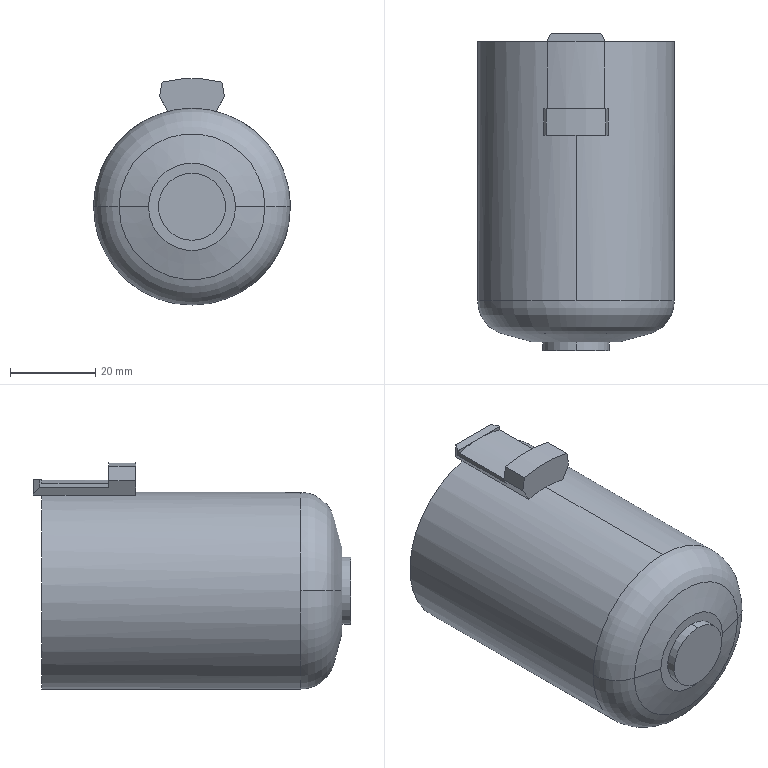Part | STEP file | _AF30-02-A_BOWL | 1 solid | 29 faces | box 46 x 74.3 x 53 mm | volume 114802 mm3 | plane 17 | cylinder 8 | torus 2 | cone 2 | commonest cylinder face diameters 46 x4 15.7 x2 52 x1 60 x1
STEP:
#1=CARTESIAN_POINT('',(23.,-92.432,0.));
#2=VERTEX_POINT('',#1);
#3=CARTESIAN_POINT('',(0.,-92.432,-23.));
#4=VERTEX_POINT('',#3);
#5=CARTESIAN_POINT('',(0.,-92.432,0.));
#6=DIRECTION('',(0.,1.,0.));
#7=DIRECTION('',(0.,0.,1.));
#8=AXIS2_PLACEMENT_3D('',#5,#6,#7);
#9=CIRCLE('',#8,23.);
#10=EDGE_CURVE('',#2,#4,#9,.T.);
#11=ORIENTED_EDGE('',*,*,#10,.T.);
#12=CARTESIAN_POINT('',(0.,-31.8,-23.));
#13=VERTEX_POINT('',#12);
#14=CARTESIAN_POINT('',(0.,-104.1,-23.));
#15=DIRECTION('',(0.,1.,0.));
#16=VECTOR('',#15,1000.);
#17=LINE('',#14,#16);
#18=EDGE_CURVE('',#4,#13,#17,.T.);
#19=ORIENTED_EDGE('',*,*,#18,.T.);
#20=CARTESIAN_POINT('',(5.604,-31.8,22.307));
#21=VERTEX_POINT('',#20);
#22=CARTESIAN_POINT('',(0.,-31.8,0.));
#23=DIRECTION('',(0.,-1.,0.));
#24=DIRECTION('',(0.,0.,1.));
#25=AXIS2_PLACEMENT_3D('',#22,#23,#24);
#26=CIRCLE('',#25,23.);
#27=EDGE_CURVE('',#13,#21,#26,.T.);
#28=ORIENTED_EDGE('',*,*,#27,.T.);
#29=CARTESIAN_POINT('',(5.604,-53.76,22.307));
#30=VERTEX_POINT('',#29);
#31=CARTESIAN_POINT('',(5.604,-104.1,22.307));
#32=DIRECTION('',(0.,-1.,0.));
#33=VECTOR('',#32,1000.);
#34=LINE('',#31,#33);
#35=EDGE_CURVE('',#21,#30,#34,.T.);
#36=ORIENTED_EDGE('',*,*,#35,.T.);
#37=CARTESIAN_POINT('',(0.,-53.76,23.));
#38=VERTEX_POINT('',#37);
#39=CARTESIAN_POINT('',(0.,-53.76,0.));
#40=DIRECTION('',(0.,-1.,0.));
#41=DIRECTION('',(0.,0.,1.));
#42=AXIS2_PLACEMENT_3D('',#39,#40,#41);
#43=CIRCLE('',#42,23.);
#44=EDGE_CURVE('',#30,#38,#43,.T.);
#45=ORIENTED_EDGE('',*,*,#44,.T.);
#46=CARTESIAN_POINT('',(0.,-92.432,23.));
#47=VERTEX_POINT('',#46);
#48=CARTESIAN_POINT('',(0.,-104.1,23.));
#49=DIRECTION('',(0.,1.,0.));
#50=VECTOR('',#49,1000.);
#51=LINE('',#48,#50);
#52=EDGE_CURVE('',#47,#38,#51,.T.);
#53=ORIENTED_EDGE('',*,*,#52,.F.);
#54=CARTESIAN_POINT('',(0.,-92.432,0.));
#55=DIRECTION('',(0.,1.,0.));
#56=DIRECTION('',(0.,0.,1.));
#57=AXIS2_PLACEMENT_3D('',#54,#55,#56);
#58=CIRCLE('',#57,23.);
#59=EDGE_CURVE('',#47,#2,#58,.T.);
#60=ORIENTED_EDGE('',*,*,#59,.T.);
#61=EDGE_LOOP('',(#11,#19,#28,#36,#45,#53,#60));
#62=FACE_OUTER_BOUND('',#61,.T.);
#63=CARTESIAN_POINT('',(0.,-104.1,0.));
#64=DIRECTION('',(0.,1.,0.));
#65=DIRECTION('',(0.,0.,1.));
#66=AXIS2_PLACEMENT_3D('',#63,#64,#65);
#67=CYLINDRICAL_SURFACE('',#66,23.);
#68=ADVANCED_FACE('',(#62),#67,.T.);
#69=CARTESIAN_POINT('',(-23.,-92.432,0.));
#70=VERTEX_POINT('',#69);
#71=CARTESIAN_POINT('',(0.,-92.432,0.));
#72=DIRECTION('',(0.,1.,0.));
#73=DIRECTION('',(0.,0.,1.));
#74=AXIS2_PLACEMENT_3D('',#71,#72,#73);
#75=CIRCLE('',#74,23.);
#76=EDGE_CURVE('',#70,#47,#75,.T.);
#77=ORIENTED_EDGE('',*,*,#76,.F.);
#78=CARTESIAN_POINT('',(-17.071,-100.159,0.));
#79=VERTEX_POINT('',#78);
#80=CARTESIAN_POINT('',(-15.,-92.432,0.));
#81=DIRECTION('',(0.,0.,1.));
#82=DIRECTION('',(1.,0.,0.));
#83=AXIS2_PLACEMENT_3D('',#80,#81,#82);
#84=CIRCLE('',#83,8.);
#85=EDGE_CURVE('',#70,#79,#84,.T.);
#86=ORIENTED_EDGE('',*,*,#85,.T.);
#87=CARTESIAN_POINT('',(17.071,-100.159,0.));
#88=VERTEX_POINT('',#87);
#89=CARTESIAN_POINT('',(0.,-100.159,0.));
#90=DIRECTION('',(0.,1.,0.));
#91=DIRECTION('',(0.,0.,-1.));
#92=AXIS2_PLACEMENT_3D('',#89,#90,#91);
#93=CIRCLE('',#92,17.071);
#94=EDGE_CURVE('',#79,#88,#93,.T.);
#95=ORIENTED_EDGE('',*,*,#94,.T.);
#96=CARTESIAN_POINT('',(15.,-92.432,0.));
#97=DIRECTION('',(0.,0.,-1.));
#98=DIRECTION('',(-1.,0.,0.));
#99=AXIS2_PLACEMENT_3D('',#96,#97,#98);
#100=CIRCLE('',#99,8.);
#101=EDGE_CURVE('',#2,#88,#100,.T.);
#102=ORIENTED_EDGE('',*,*,#101,.F.);
#103=ORIENTED_EDGE('',*,*,#59,.F.);
#104=EDGE_LOOP('',(#77,#86,#95,#102,#103));
#105=FACE_OUTER_BOUND('',#104,.T.);
#106=CARTESIAN_POINT('',(0.,-92.432,0.));
#107=DIRECTION('',(0.,-1.,0.));
#108=DIRECTION('',(1.,0.,0.));
#109=AXIS2_PLACEMENT_3D('',#106,#107,#108);
#110=TOROIDAL_SURFACE('',#109,15.,8.);
#111=ADVANCED_FACE('',(#105),#110,.T.);
#112=CARTESIAN_POINT('',(0.,-31.8,23.));
#113=VERTEX_POINT('',#112);
#114=CARTESIAN_POINT('',(0.,-31.8,0.));
#115=DIRECTION('',(0.,-1.,0.));
#116=DIRECTION('',(0.,0.,1.));
#117=AXIS2_PLACEMENT_3D('',#114,#115,#116);
#118=CIRCLE('',#117,23.);
#119=EDGE_CURVE('',#21,#113,#118,.T.);
#120=ORIENTED_EDGE('',*,*,#119,.T.);
#121=CARTESIAN_POINT('',(0.,-29.8,23.));
#122=VERTEX_POINT('',#121);
#123=CARTESIAN_POINT('',(0.,-29.8,23.));
#124=DIRECTION('',(0.,1.,0.));
#125=VECTOR('',#124,1000.);
#126=LINE('',#123,#125);
#127=EDGE_CURVE('',#113,#122,#126,.T.);
#128=ORIENTED_EDGE('',*,*,#127,.T.);
#129=CARTESIAN_POINT('',(5.604,-29.8,22.307));
#130=VERTEX_POINT('',#129);
#131=CARTESIAN_POINT('',(0.,-29.8,0.));
#132=DIRECTION('',(0.,-1.,0.));
#133=DIRECTION('',(0.,0.,1.));
#134=AXIS2_PLACEMENT_3D('',#131,#132,#133);
#135=CIRCLE('',#134,23.);
#136=EDGE_CURVE('',#130,#122,#135,.T.);
#137=ORIENTED_EDGE('',*,*,#136,.F.);
#138=CARTESIAN_POINT('',(5.604,-47.45,22.307));
#139=DIRECTION('',(0.,1.,0.));
#140=VECTOR('',#139,1000.);
#141=LINE('',#138,#140);
#142=EDGE_CURVE('',#21,#130,#141,.T.);
#143=ORIENTED_EDGE('',*,*,#142,.F.);
#144=EDGE_LOOP('',(#120,#128,#137,#143));
#145=FACE_OUTER_BOUND('',#144,.T.);
#146=CARTESIAN_POINT('',(0.,-29.8,0.));
#147=DIRECTION('',(0.,1.,0.));
#148=DIRECTION('',(0.,0.,1.));
#149=AXIS2_PLACEMENT_3D('',#146,#147,#148);
#150=CYLINDRICAL_SURFACE('',#149,23.);
#151=ADVANCED_FACE('',(#145),#150,.F.);
#152=CARTESIAN_POINT('',(-10.2,-102.,0.));
#153=VERTEX_POINT('',#152);
#154=CARTESIAN_POINT('',(10.2,-102.,0.));
#155=VERTEX_POINT('',#154);
#156=CARTESIAN_POINT('',(0.,-102.,0.));
#157=DIRECTION('',(0.,1.,0.));
#158=DIRECTION('',(-1.,0.,0.));
#159=AXIS2_PLACEMENT_3D('',#156,#157,#158);
#160=CIRCLE('',#159,10.2);
#161=EDGE_CURVE('',#153,#155,#160,.T.);
#162=ORIENTED_EDGE('',*,*,#161,.T.);
#163=CARTESIAN_POINT('',(17.071,-100.159,0.));
#164=DIRECTION('',(0.9659,0.2588,0.));
#165=VECTOR('',#164,1000.);
#166=LINE('',#163,#165);
#167=EDGE_CURVE('',#155,#88,#166,.T.);
#168=ORIENTED_EDGE('',*,*,#167,.T.);
#169=ORIENTED_EDGE('',*,*,#94,.F.);
#170=CARTESIAN_POINT('',(-17.071,-100.159,0.));
#171=DIRECTION('',(-0.9659,0.2588,0.));
#172=VECTOR('',#171,1000.);
#173=LINE('',#170,#172);
#174=EDGE_CURVE('',#153,#79,#173,.T.);
#175=ORIENTED_EDGE('',*,*,#174,.F.);
#176=EDGE_LOOP('',(#162,#168,#169,#175));
#177=FACE_OUTER_BOUND('',#176,.T.);
#178=CARTESIAN_POINT('',(0.,-100.159,0.));
#179=DIRECTION('',(0.,1.,0.));
#180=DIRECTION('',(-1.,0.,0.));
#181=AXIS2_PLACEMENT_3D('',#178,#179,#180);
#182=CONICAL_SURFACE('',#181,17.071,1.309);
#183=ADVANCED_FACE('',(#177),#182,.T.);
#184=CARTESIAN_POINT('',(0.,-104.1,7.85));
#185=VERTEX_POINT('',#184);
#186=CARTESIAN_POINT('',(0.,-104.1,-7.85));
#187=VERTEX_POINT('',#186);
#188=CARTESIAN_POINT('',(0.,-104.1,0.));
#189=DIRECTION('',(0.,1.,0.));
#190=DIRECTION('',(0.,0.,1.));
#191=AXIS2_PLACEMENT_3D('',#188,#189,#190);
#192=CIRCLE('',#191,7.85);
#193=EDGE_CURVE('',#185,#187,#192,.T.);
#194=ORIENTED_EDGE('',*,*,#193,.T.);
#195=CARTESIAN_POINT('',(0.,-102.,-7.85));
#196=VERTEX_POINT('',#195);
#197=CARTESIAN_POINT('',(0.,-104.1,-7.85));
#198=DIRECTION('',(0.,1.,0.));
#199=VECTOR('',#198,1000.);
#200=LINE('',#197,#199);
#201=EDGE_CURVE('',#187,#196,#200,.T.);
#202=ORIENTED_EDGE('',*,*,#201,.T.);
#203=CARTESIAN_POINT('',(0.,-102.,7.85));
#204=VERTEX_POINT('',#203);
#205=CARTESIAN_POINT('',(0.,-102.,0.));
#206=DIRECTION('',(0.,-1.,0.));
#207=DIRECTION('',(0.,0.,1.));
#208=AXIS2_PLACEMENT_3D('',#205,#206,#207);
#209=CIRCLE('',#208,7.85);
#210=EDGE_CURVE('',#196,#204,#209,.T.);
#211=ORIENTED_EDGE('',*,*,#210,.T.);
#212=CARTESIAN_POINT('',(0.,-104.1,7.85));
#213=DIRECTION('',(0.,1.,0.));
#214=VECTOR('',#213,1000.);
#215=LINE('',#212,#214);
#216=EDGE_CURVE('',#185,#204,#215,.T.);
#217=ORIENTED_EDGE('',*,*,#216,.F.);
#218=EDGE_LOOP('',(#194,#202,#211,#217));
#219=FACE_OUTER_BOUND('',#218,.T.);
#220=CARTESIAN_POINT('',(0.,-104.1,0.));
#221=DIRECTION('',(0.,1.,0.));
#222=DIRECTION('',(0.,0.,1.));
#223=AXIS2_PLACEMENT_3D('',#220,#221,#222);
#224=CYLINDRICAL_SURFACE('',#223,7.85);
#225=ADVANCED_FACE('',(#219),#224,.T.);
#226=ORIENTED_EDGE('',*,*,#18,.F.);
#227=CARTESIAN_POINT('',(0.,-92.432,0.));
#228=DIRECTION('',(0.,1.,0.));
#229=DIRECTION('',(0.,0.,1.));
#230=AXIS2_PLACEMENT_3D('',#227,#228,#229);
#231=CIRCLE('',#230,23.);
#232=EDGE_CURVE('',#4,#70,#231,.T.);
#233=ORIENTED_EDGE('',*,*,#232,.T.);
#234=ORIENTED_EDGE('',*,*,#76,.T.);
#235=ORIENTED_EDGE('',*,*,#52,.T.);
#236=CARTESIAN_POINT('',(-5.604,-53.76,22.307));
#237=VERTEX_POINT('',#236);
#238=CARTESIAN_POINT('',(0.,-53.76,0.));
#239=DIRECTION('',(0.,-1.,0.));
#240=DIRECTION('',(0.,0.,1.));
#241=AXIS2_PLACEMENT_3D('',#238,#239,#240);
#242=CIRCLE('',#241,23.);
#243=EDGE_CURVE('',#38,#237,#242,.T.);
#244=ORIENTED_EDGE('',*,*,#243,.T.);
#245=CARTESIAN_POINT('',(-5.604,-31.8,22.307));
#246=VERTEX_POINT('',#245);
#247=CARTESIAN_POINT('',(-5.604,-104.1,22.307));
#248=DIRECTION('',(0.,1.,0.));
#249=VECTOR('',#248,1000.);
#250=LINE('',#247,#249);
#251=EDGE_CURVE('',#237,#246,#250,.T.);
#252=ORIENTED_EDGE('',*,*,#251,.T.);
#253=CARTESIAN_POINT('',(0.,-31.8,0.));
#254=DIRECTION('',(0.,-1.,0.));
#255=DIRECTION('',(0.,0.,1.));
#256=AXIS2_PLACEMENT_3D('',#253,#254,#255);
#257=CIRCLE('',#256,23.);
#258=EDGE_CURVE('',#246,#13,#257,.T.);
#259=ORIENTED_EDGE('',*,*,#258,.T.);
#260=EDGE_LOOP('',(#226,#233,#234,#235,#244,#252,#259));
#261=FACE_OUTER_BOUND('',#260,.T.);
#262=CARTESIAN_POINT('',(0.,-104.1,0.));
#263=DIRECTION('',(0.,1.,0.));
#264=DIRECTION('',(0.,0.,1.));
#265=AXIS2_PLACEMENT_3D('',#262,#263,#264);
#266=CYLINDRICAL_SURFACE('',#265,23.);
#267=ADVANCED_FACE('',(#261),#266,.T.);
#268=CARTESIAN_POINT('',(7.6,-53.76,25.765));
#269=VERTEX_POINT('',#268);
#270=CARTESIAN_POINT('',(7.6,-53.76,25.765));
#271=DIRECTION('',(-0.5,0.,-0.866));
#272=VECTOR('',#271,1000.);
#273=LINE('',#270,#272);
#274=EDGE_CURVE('',#269,#30,#273,.T.);
#275=ORIENTED_EDGE('',*,*,#274,.F.);
#276=CARTESIAN_POINT('',(7.004,-53.76,29.171));
#277=VERTEX_POINT('',#276);
#278=CARTESIAN_POINT('',(7.004,-53.76,29.171));
#279=DIRECTION('',(0.1723,0.,-0.985));
#280=VECTOR('',#279,1000.);
#281=LINE('',#278,#280);
#282=EDGE_CURVE('',#277,#269,#281,.T.);
#283=ORIENTED_EDGE('',*,*,#282,.F.);
#284=CARTESIAN_POINT('',(-7.004,-53.76,29.171));
#285=VERTEX_POINT('',#284);
#286=CARTESIAN_POINT('',(0.,-53.76,0.));
#287=DIRECTION('',(0.,1.,0.));
#288=DIRECTION('',(0.,0.,-1.));
#289=AXIS2_PLACEMENT_3D('',#286,#287,#288);
#290=CIRCLE('',#289,30.);
#291=EDGE_CURVE('',#285,#277,#290,.T.);
#292=ORIENTED_EDGE('',*,*,#291,.F.);
#293=CARTESIAN_POINT('',(-7.6,-53.76,25.765));
#294=VERTEX_POINT('',#293);
#295=CARTESIAN_POINT('',(-7.6,-53.76,25.765));
#296=DIRECTION('',(0.1723,0.,0.985));
#297=VECTOR('',#296,1000.);
#298=LINE('',#295,#297);
#299=EDGE_CURVE('',#294,#285,#298,.T.);
#300=ORIENTED_EDGE('',*,*,#299,.F.);
#301=CARTESIAN_POINT('',(-5.604,-53.76,22.307));
#302=DIRECTION('',(-0.5,0.,0.866));
#303=VECTOR('',#302,1000.);
#304=LINE('',#301,#303);
#305=EDGE_CURVE('',#237,#294,#304,.T.);
#306=ORIENTED_EDGE('',*,*,#305,.F.);
#307=ORIENTED_EDGE('',*,*,#243,.F.);
#308=ORIENTED_EDGE('',*,*,#44,.F.);
#309=EDGE_LOOP('',(#275,#283,#292,#300,#306,#307,#308));
#310=FACE_OUTER_BOUND('',#309,.T.);
#311=CARTESIAN_POINT('',(0.,-53.76,0.));
#312=DIRECTION('',(0.,1.,0.));
#313=DIRECTION('',(0.,0.,1.));
#314=AXIS2_PLACEMENT_3D('',#311,#312,#313);
#315=PLANE('',#314);
#316=ADVANCED_FACE('',(#310),#315,.F.);
#317=CARTESIAN_POINT('',(7.6,-47.45,25.765));
#318=VERTEX_POINT('',#317);
#319=CARTESIAN_POINT('',(7.6,-47.45,25.765));
#320=DIRECTION('',(0.,-1.,0.));
#321=VECTOR('',#320,1000.);
#322=LINE('',#319,#321);
#323=EDGE_CURVE('',#318,#269,#322,.T.);
#324=ORIENTED_EDGE('',*,*,#323,.T.);
#325=ORIENTED_EDGE('',*,*,#274,.T.);
#326=ORIENTED_EDGE('',*,*,#35,.F.);
#327=ORIENTED_EDGE('',*,*,#142,.T.);
#328=CARTESIAN_POINT('',(5.798,-29.8,22.644));
#329=VERTEX_POINT('',#328);
#330=CARTESIAN_POINT('',(5.798,-29.8,22.644));
#331=DIRECTION('',(-0.5,0.,-0.866));
#332=VECTOR('',#331,1000.);
#333=LINE('',#330,#332);
#334=EDGE_CURVE('',#329,#130,#333,.T.);
#335=ORIENTED_EDGE('',*,*,#334,.F.);
#336=CARTESIAN_POINT('',(6.7,-31.301,24.206));
#337=VERTEX_POINT('',#336);
#338=CARTESIAN_POINT('',(5.798,-29.8,22.644));
#339=DIRECTION('',(0.3843,-0.6396,0.6657));
#340=VECTOR('',#339,1000.);
#341=LINE('',#338,#340);
#342=EDGE_CURVE('',#329,#337,#341,.T.);
#343=ORIENTED_EDGE('',*,*,#342,.T.);
#344=CARTESIAN_POINT('',(6.7,-47.45,24.206));
#345=VERTEX_POINT('',#344);
#346=CARTESIAN_POINT('',(6.7,-47.45,24.206));
#347=DIRECTION('',(0.,-1.,0.));
#348=VECTOR('',#347,1000.);
#349=LINE('',#346,#348);
#350=EDGE_CURVE('',#337,#345,#349,.T.);
#351=ORIENTED_EDGE('',*,*,#350,.T.);
#352=CARTESIAN_POINT('',(6.7,-47.45,24.206));
#353=DIRECTION('',(0.5,0.,0.866));
#354=VECTOR('',#353,1000.);
#355=LINE('',#352,#354);
#356=EDGE_CURVE('',#345,#318,#355,.T.);
#357=ORIENTED_EDGE('',*,*,#356,.T.);
#358=EDGE_LOOP('',(#324,#325,#326,#327,#335,#343,#351,#357));
#359=FACE_OUTER_BOUND('',#358,.T.);
#360=CARTESIAN_POINT('',(6.7,-47.45,24.206));
#361=DIRECTION('',(0.866,0.,-0.5));
#362=DIRECTION('',(-0.5,0.,-0.866));
#363=AXIS2_PLACEMENT_3D('',#360,#361,#362);
#364=PLANE('',#363);
#365=ADVANCED_FACE('',(#359),#364,.T.);
#366=ORIENTED_EDGE('',*,*,#258,.F.);
#367=CARTESIAN_POINT('',(0.,-31.8,0.));
#368=DIRECTION('',(0.,-1.,0.));
#369=DIRECTION('',(0.,0.,1.));
#370=AXIS2_PLACEMENT_3D('',#367,#368,#369);
#371=CIRCLE('',#370,23.);
#372=EDGE_CURVE('',#113,#246,#371,.T.);
#373=ORIENTED_EDGE('',*,*,#372,.F.);
#374=ORIENTED_EDGE('',*,*,#119,.F.);
#375=ORIENTED_EDGE('',*,*,#27,.F.);
#376=EDGE_LOOP('',(#366,#373,#374,#375));
#377=FACE_OUTER_BOUND('',#376,.T.);
#378=CARTESIAN_POINT('',(0.,-31.8,0.));
#379=DIRECTION('',(0.,-1.,0.));
#380=DIRECTION('',(0.,0.,-1.));
#381=AXIS2_PLACEMENT_3D('',#378,#379,#380);
#382=PLANE('',#381);
#383=ADVANCED_FACE('',(#377),#382,.F.);
#384=ORIENTED_EDGE('',*,*,#85,.F.);
#385=ORIENTED_EDGE('',*,*,#232,.F.);
#386=ORIENTED_EDGE('',*,*,#10,.F.);
#387=ORIENTED_EDGE('',*,*,#101,.T.);
#388=CARTESIAN_POINT('',(0.,-100.159,0.));
#389=DIRECTION('',(0.,1.,0.));
#390=DIRECTION('',(0.,0.,-1.));
#391=AXIS2_PLACEMENT_3D('',#388,#389,#390);
#392=CIRCLE('',#391,17.071);
#393=EDGE_CURVE('',#88,#79,#392,.T.);
#394=ORIENTED_EDGE('',*,*,#393,.T.);
#395=EDGE_LOOP('',(#384,#385,#386,#387,#394));
#396=FACE_OUTER_BOUND('',#395,.T.);
#397=CARTESIAN_POINT('',(0.,-92.432,0.));
#398=DIRECTION('',(0.,-1.,0.));
#399=DIRECTION('',(1.,0.,0.));
#400=AXIS2_PLACEMENT_3D('',#397,#398,#399);
#401=TOROIDAL_SURFACE('',#400,15.,8.);
#402=ADVANCED_FACE('',(#396),#401,.T.);
#403=ORIENTED_EDGE('',*,*,#251,.F.);
#404=ORIENTED_EDGE('',*,*,#305,.T.);
#405=CARTESIAN_POINT('',(-7.6,-47.45,25.765));
#406=VERTEX_POINT('',#405);
#407=CARTESIAN_POINT('',(-7.6,-47.45,25.765));
#408=DIRECTION('',(0.,1.,0.));
#409=VECTOR('',#408,1000.);
#410=LINE('',#407,#409);
#411=EDGE_CURVE('',#294,#406,#410,.T.);
#412=ORIENTED_EDGE('',*,*,#411,.T.);
#413=CARTESIAN_POINT('',(-6.7,-47.45,24.206));
#414=VERTEX_POINT('',#413);
#415=CARTESIAN_POINT('',(-5.541,-47.45,22.199));
#416=DIRECTION('',(0.5,0.,-0.866));
#417=VECTOR('',#416,1000.);
#418=LINE('',#415,#417);
#419=EDGE_CURVE('',#406,#414,#418,.T.);
#420=ORIENTED_EDGE('',*,*,#419,.T.);
#421=CARTESIAN_POINT('',(-6.7,-31.301,24.206));
#422=VERTEX_POINT('',#421);
#423=CARTESIAN_POINT('',(-6.7,-47.45,24.206));
#424=DIRECTION('',(0.,1.,0.));
#425=VECTOR('',#424,1000.);
#426=LINE('',#423,#425);
#427=EDGE_CURVE('',#414,#422,#426,.T.);
#428=ORIENTED_EDGE('',*,*,#427,.T.);
#429=CARTESIAN_POINT('',(-5.798,-29.8,22.644));
#430=VERTEX_POINT('',#429);
#431=CARTESIAN_POINT('',(-6.7,-31.301,24.206));
#432=DIRECTION('',(0.3843,0.6396,-0.6657));
#433=VECTOR('',#432,1000.);
#434=LINE('',#431,#433);
#435=EDGE_CURVE('',#422,#430,#434,.T.);
#436=ORIENTED_EDGE('',*,*,#435,.T.);
#437=CARTESIAN_POINT('',(-5.604,-29.8,22.307));
#438=VERTEX_POINT('',#437);
#439=CARTESIAN_POINT('',(-5.604,-29.8,22.307));
#440=DIRECTION('',(-0.5,0.,0.866));
#441=VECTOR('',#440,1000.);
#442=LINE('',#439,#441);
#443=EDGE_CURVE('',#438,#430,#442,.T.);
#444=ORIENTED_EDGE('',*,*,#443,.F.);
#445=CARTESIAN_POINT('',(-5.604,-47.45,22.307));
#446=DIRECTION('',(0.,-1.,0.));
#447=VECTOR('',#446,1000.);
#448=LINE('',#445,#447);
#449=EDGE_CURVE('',#438,#246,#448,.T.);
#450=ORIENTED_EDGE('',*,*,#449,.T.);
#451=EDGE_LOOP('',(#403,#404,#412,#420,#428,#436,#444,#450));
#452=FACE_OUTER_BOUND('',#451,.T.);
#453=CARTESIAN_POINT('',(-5.541,-47.45,22.199));
#454=DIRECTION('',(-0.866,0.,-0.5));
#455=DIRECTION('',(-0.5,0.,0.866));
#456=AXIS2_PLACEMENT_3D('',#453,#454,#455);
#457=PLANE('',#456);
#458=ADVANCED_FACE('',(#452),#457,.T.);
#459=CARTESIAN_POINT('',(7.004,-47.45,29.171));
#460=VERTEX_POINT('',#459);
#461=CARTESIAN_POINT('',(7.004,-47.45,29.171));
#462=DIRECTION('',(-0.1723,0.,0.985));
#463=VECTOR('',#462,1000.);
#464=LINE('',#461,#463);
#465=EDGE_CURVE('',#318,#460,#464,.T.);
#466=ORIENTED_EDGE('',*,*,#465,.T.);
#467=CARTESIAN_POINT('',(7.004,-53.76,29.171));
#468=DIRECTION('',(0.,-1.,0.));
#469=VECTOR('',#468,1000.);
#470=LINE('',#467,#469);
#471=EDGE_CURVE('',#460,#277,#470,.T.);
#472=ORIENTED_EDGE('',*,*,#471,.T.);
#473=ORIENTED_EDGE('',*,*,#282,.T.);
#474=ORIENTED_EDGE('',*,*,#323,.F.);
#475=EDGE_LOOP('',(#466,#472,#473,#474));
#476=FACE_OUTER_BOUND('',#475,.T.);
#477=CARTESIAN_POINT('',(7.004,-53.76,29.171));
#478=DIRECTION('',(0.985,0.,0.1723));
#479=DIRECTION('',(0.1723,0.,-0.985));
#480=AXIS2_PLACEMENT_3D('',#477,#478,#479);
#481=PLANE('',#480);
#482=ADVANCED_FACE('',(#476),#481,.T.);
#483=CARTESIAN_POINT('',(-7.004,-47.45,29.171));
#484=VERTEX_POINT('',#483);
#485=CARTESIAN_POINT('',(0.,-47.45,0.));
#486=DIRECTION('',(0.,-1.,0.));
#487=DIRECTION('',(0.,0.,-1.));
#488=AXIS2_PLACEMENT_3D('',#485,#486,#487);
#489=CIRCLE('',#488,30.);
#490=EDGE_CURVE('',#460,#484,#489,.T.);
#491=ORIENTED_EDGE('',*,*,#490,.T.);
#492=CARTESIAN_POINT('',(-7.004,-53.76,29.171));
#493=DIRECTION('',(0.,-1.,0.));
#494=VECTOR('',#493,1000.);
#495=LINE('',#492,#494);
#496=EDGE_CURVE('',#484,#285,#495,.T.);
#497=ORIENTED_EDGE('',*,*,#496,.T.);
#498=ORIENTED_EDGE('',*,*,#291,.T.);
#499=ORIENTED_EDGE('',*,*,#471,.F.);
#500=EDGE_LOOP('',(#491,#497,#498,#499));
#501=FACE_OUTER_BOUND('',#500,.T.);
#502=CARTESIAN_POINT('',(0.,-53.76,0.));
#503=DIRECTION('',(0.,-1.,0.));
#504=DIRECTION('',(0.,0.,-1.));
#505=AXIS2_PLACEMENT_3D('',#502,#503,#504);
#506=CYLINDRICAL_SURFACE('',#505,30.);
#507=ADVANCED_FACE('',(#501),#506,.T.);
#508=CARTESIAN_POINT('',(-7.6,-47.45,25.765));
#509=DIRECTION('',(-0.1723,0.,-0.985));
#510=VECTOR('',#509,1000.);
#511=LINE('',#508,#510);
#512=EDGE_CURVE('',#484,#406,#511,.T.);
#513=ORIENTED_EDGE('',*,*,#512,.T.);
#514=ORIENTED_EDGE('',*,*,#411,.F.);
#515=ORIENTED_EDGE('',*,*,#299,.T.);
#516=ORIENTED_EDGE('',*,*,#496,.F.);
#517=EDGE_LOOP('',(#513,#514,#515,#516));
#518=FACE_OUTER_BOUND('',#517,.T.);
#519=CARTESIAN_POINT('',(-7.6,-53.76,25.765));
#520=DIRECTION('',(-0.985,0.,0.1723));
#521=DIRECTION('',(0.1723,0.,0.985));
#522=AXIS2_PLACEMENT_3D('',#519,#520,#521);
#523=PLANE('',#522);
#524=ADVANCED_FACE('',(#518),#523,.T.);
#525=ORIENTED_EDGE('',*,*,#490,.F.);
#526=ORIENTED_EDGE('',*,*,#465,.F.);
#527=ORIENTED_EDGE('',*,*,#356,.F.);
#528=CARTESIAN_POINT('',(6.7,-47.45,25.122));
#529=VERTEX_POINT('',#528);
#530=CARTESIAN_POINT('',(6.7,-47.45,0.));
#531=DIRECTION('',(0.,0.,1.));
#532=VECTOR('',#531,1000.);
#533=LINE('',#530,#532);
#534=EDGE_CURVE('',#345,#529,#533,.T.);
#535=ORIENTED_EDGE('',*,*,#534,.T.);
#536=CARTESIAN_POINT('',(-6.7,-47.45,25.122));
#537=VERTEX_POINT('',#536);
#538=CARTESIAN_POINT('',(0.,-47.45,0.));
#539=DIRECTION('',(0.,-1.,0.));
#540=DIRECTION('',(0.,0.,-1.));
#541=AXIS2_PLACEMENT_3D('',#538,#539,#540);
#542=CIRCLE('',#541,26.);
#543=EDGE_CURVE('',#529,#537,#542,.T.);
#544=ORIENTED_EDGE('',*,*,#543,.T.);
#545=CARTESIAN_POINT('',(-6.7,-47.45,0.));
#546=DIRECTION('',(0.,0.,-1.));
#547=VECTOR('',#546,1000.);
#548=LINE('',#545,#547);
#549=EDGE_CURVE('',#537,#414,#548,.T.);
#550=ORIENTED_EDGE('',*,*,#549,.T.);
#551=ORIENTED_EDGE('',*,*,#419,.F.);
#552=ORIENTED_EDGE('',*,*,#512,.F.);
#553=EDGE_LOOP('',(#525,#526,#527,#535,#544,#550,#551,#552));
#554=FACE_OUTER_BOUND('',#553,.T.);
#555=CARTESIAN_POINT('',(0.,-47.45,0.));
#556=DIRECTION('',(0.,1.,0.));
#557=DIRECTION('',(0.,0.,1.));
#558=AXIS2_PLACEMENT_3D('',#555,#556,#557);
#559=PLANE('',#558);
#560=ADVANCED_FACE('',(#554),#559,.T.);
#561=CARTESIAN_POINT('',(6.7,-31.301,26.));
#562=VERTEX_POINT('',#561);
#563=CARTESIAN_POINT('',(6.7,-31.8,26.));
#564=VERTEX_POINT('',#563);
#565=CARTESIAN_POINT('',(6.7,-29.8,26.));
#566=DIRECTION('',(0.,-1.,0.));
#567=VECTOR('',#566,1000.);
#568=LINE('',#565,#567);
#569=EDGE_CURVE('',#562,#564,#568,.T.);
#570=ORIENTED_EDGE('',*,*,#569,.T.);
#571=CARTESIAN_POINT('',(6.7,-31.8,25.122));
#572=VERTEX_POINT('',#571);
#573=CARTESIAN_POINT('',(6.7,-31.8,0.));
#574=DIRECTION('',(0.,0.,-1.));
#575=VECTOR('',#574,1000.);
#576=LINE('',#573,#575);
#577=EDGE_CURVE('',#564,#572,#576,.T.);
#578=ORIENTED_EDGE('',*,*,#577,.T.);
#579=CARTESIAN_POINT('',(6.7,-47.45,25.122));
#580=DIRECTION('',(0.,-1.,0.));
#581=VECTOR('',#580,1000.);
#582=LINE('',#579,#581);
#583=EDGE_CURVE('',#572,#529,#582,.T.);
#584=ORIENTED_EDGE('',*,*,#583,.T.);
#585=ORIENTED_EDGE('',*,*,#534,.F.);
#586=ORIENTED_EDGE('',*,*,#350,.F.);
#587=CARTESIAN_POINT('',(6.7,-31.301,25.122));
#588=DIRECTION('',(0.,0.,1.));
#589=VECTOR('',#588,1000.);
#590=LINE('',#587,#589);
#591=EDGE_CURVE('',#337,#562,#590,.T.);
#592=ORIENTED_EDGE('',*,*,#591,.T.);
#593=EDGE_LOOP('',(#570,#578,#584,#585,#586,#592));
#594=FACE_OUTER_BOUND('',#593,.T.);
#595=CARTESIAN_POINT('',(6.7,-47.45,25.122));
#596=DIRECTION('',(1.,0.,0.));
#597=DIRECTION('',(0.,0.,-1.));
#598=AXIS2_PLACEMENT_3D('',#595,#596,#597);
#599=PLANE('',#598);
#600=ADVANCED_FACE('',(#594),#599,.T.);
#601=CARTESIAN_POINT('',(5.798,-29.8,26.));
#602=VERTEX_POINT('',#601);
#603=CARTESIAN_POINT('',(5.798,-29.8,28.));
#604=DIRECTION('',(0.,0.,1.));
#605=VECTOR('',#604,1000.);
#606=LINE('',#603,#605);
#607=EDGE_CURVE('',#329,#602,#606,.T.);
#608=ORIENTED_EDGE('',*,*,#607,.T.);
#609=CARTESIAN_POINT('',(5.798,-29.8,26.));
#610=DIRECTION('',(0.515,-0.8572,0.));
#611=VECTOR('',#610,1000.);
#612=LINE('',#609,#611);
#613=EDGE_CURVE('',#602,#562,#612,.T.);
#614=ORIENTED_EDGE('',*,*,#613,.T.);
#615=ORIENTED_EDGE('',*,*,#591,.F.);
#616=ORIENTED_EDGE('',*,*,#342,.F.);
#617=EDGE_LOOP('',(#608,#614,#615,#616));
#618=FACE_OUTER_BOUND('',#617,.T.);
#619=CARTESIAN_POINT('',(5.798,-29.8,28.));
#620=DIRECTION('',(0.8572,0.515,0.));
#621=DIRECTION('',(-0.515,0.8572,0.));
#622=AXIS2_PLACEMENT_3D('',#619,#620,#621);
#623=PLANE('',#622);
#624=ADVANCED_FACE('',(#618),#623,.T.);
#625=ORIENTED_EDGE('',*,*,#127,.F.);
#626=ORIENTED_EDGE('',*,*,#372,.T.);
#627=ORIENTED_EDGE('',*,*,#449,.F.);
#628=CARTESIAN_POINT('',(0.,-29.8,0.));
#629=DIRECTION('',(0.,-1.,0.));
#630=DIRECTION('',(0.,0.,1.));
#631=AXIS2_PLACEMENT_3D('',#628,#629,#630);
#632=CIRCLE('',#631,23.);
#633=EDGE_CURVE('',#122,#438,#632,.T.);
#634=ORIENTED_EDGE('',*,*,#633,.F.);
#635=EDGE_LOOP('',(#625,#626,#627,#634));
#636=FACE_OUTER_BOUND('',#635,.T.);
#637=CARTESIAN_POINT('',(0.,-29.8,0.));
#638=DIRECTION('',(0.,1.,0.));
#639=DIRECTION('',(0.,0.,1.));
#640=AXIS2_PLACEMENT_3D('',#637,#638,#639);
#641=CYLINDRICAL_SURFACE('',#640,23.);
#642=ADVANCED_FACE('',(#636),#641,.F.);
#643=ORIENTED_EDGE('',*,*,#167,.F.);
#644=CARTESIAN_POINT('',(0.,-102.,0.));
#645=DIRECTION('',(0.,1.,0.));
#646=DIRECTION('',(-1.,0.,0.));
#647=AXIS2_PLACEMENT_3D('',#644,#645,#646);
#648=CIRCLE('',#647,10.2);
#649=EDGE_CURVE('',#155,#153,#648,.T.);
#650=ORIENTED_EDGE('',*,*,#649,.T.);
#651=ORIENTED_EDGE('',*,*,#174,.T.);
#652=ORIENTED_EDGE('',*,*,#393,.F.);
#653=EDGE_LOOP('',(#643,#650,#651,#652));
#654=FACE_OUTER_BOUND('',#653,.T.);
#655=CARTESIAN_POINT('',(0.,-100.159,0.));
#656=DIRECTION('',(0.,1.,0.));
#657=DIRECTION('',(-1.,0.,0.));
#658=AXIS2_PLACEMENT_3D('',#655,#656,#657);
#659=CONICAL_SURFACE('',#658,17.071,1.309);
#660=ADVANCED_FACE('',(#654),#659,.T.);
#661=CARTESIAN_POINT('',(-6.7,-31.301,26.));
#662=VERTEX_POINT('',#661);
#663=CARTESIAN_POINT('',(-6.7,-31.301,28.));
#664=DIRECTION('',(0.,0.,1.));
#665=VECTOR('',#664,1000.);
#666=LINE('',#663,#665);
#667=EDGE_CURVE('',#422,#662,#666,.T.);
#668=ORIENTED_EDGE('',*,*,#667,.T.);
#669=CARTESIAN_POINT('',(-5.798,-29.8,26.));
#670=VERTEX_POINT('',#669);
#671=CARTESIAN_POINT('',(-7.,-31.8,26.));
#672=DIRECTION('',(0.515,0.8572,0.));
#673=VECTOR('',#672,1000.);
#674=LINE('',#671,#673);
#675=EDGE_CURVE('',#662,#670,#674,.T.);
#676=ORIENTED_EDGE('',*,*,#675,.T.);
#677=CARTESIAN_POINT('',(-5.798,-29.8,28.));
#678=DIRECTION('',(0.,0.,-1.));
#679=VECTOR('',#678,1000.);
#680=LINE('',#677,#679);
#681=EDGE_CURVE('',#670,#430,#680,.T.);
#682=ORIENTED_EDGE('',*,*,#681,.T.);
#683=ORIENTED_EDGE('',*,*,#435,.F.);
#684=EDGE_LOOP('',(#668,#676,#682,#683));
#685=FACE_OUTER_BOUND('',#684,.T.);
#686=CARTESIAN_POINT('',(-7.,-31.8,28.));
#687=DIRECTION('',(-0.8572,0.515,0.));
#688=DIRECTION('',(-0.515,-0.8572,0.));
#689=AXIS2_PLACEMENT_3D('',#686,#687,#688);
#690=PLANE('',#689);
#691=ADVANCED_FACE('',(#685),#690,.T.);
#692=ORIENTED_EDGE('',*,*,#427,.F.);
#693=ORIENTED_EDGE('',*,*,#549,.F.);
#694=CARTESIAN_POINT('',(-6.7,-31.8,25.122));
#695=VERTEX_POINT('',#694);
#696=CARTESIAN_POINT('',(-6.7,-47.45,25.122));
#697=DIRECTION('',(0.,1.,0.));
#698=VECTOR('',#697,1000.);
#699=LINE('',#696,#698);
#700=EDGE_CURVE('',#537,#695,#699,.T.);
#701=ORIENTED_EDGE('',*,*,#700,.T.);
#702=CARTESIAN_POINT('',(-6.7,-31.8,26.));
#703=VERTEX_POINT('',#702);
#704=CARTESIAN_POINT('',(-6.7,-31.8,0.));
#705=DIRECTION('',(0.,0.,1.));
#706=VECTOR('',#705,1000.);
#707=LINE('',#704,#706);
#708=EDGE_CURVE('',#695,#703,#707,.T.);
#709=ORIENTED_EDGE('',*,*,#708,.T.);
#710=CARTESIAN_POINT('',(-6.7,-47.45,26.));
#711=DIRECTION('',(0.,1.,0.));
#712=VECTOR('',#711,1000.);
#713=LINE('',#710,#712);
#714=EDGE_CURVE('',#703,#662,#713,.T.);
#715=ORIENTED_EDGE('',*,*,#714,.T.);
#716=ORIENTED_EDGE('',*,*,#667,.F.);
#717=EDGE_LOOP('',(#692,#693,#701,#709,#715,#716));
#718=FACE_OUTER_BOUND('',#717,.T.);
#719=CARTESIAN_POINT('',(-6.7,-47.45,24.206));
#720=DIRECTION('',(-1.,0.,0.));
#721=DIRECTION('',(0.,0.,1.));
#722=AXIS2_PLACEMENT_3D('',#719,#720,#721);
#723=PLANE('',#722);
#724=ADVANCED_FACE('',(#718),#723,.T.);
#725=ORIENTED_EDGE('',*,*,#700,.F.);
#726=ORIENTED_EDGE('',*,*,#543,.F.);
#727=ORIENTED_EDGE('',*,*,#583,.F.);
#728=CARTESIAN_POINT('',(0.,-31.8,26.));
#729=VERTEX_POINT('',#728);
#730=CARTESIAN_POINT('',(0.,-31.8,0.));
#731=DIRECTION('',(0.,-1.,0.));
#732=DIRECTION('',(0.,0.,-1.));
#733=AXIS2_PLACEMENT_3D('',#730,#731,#732);
#734=CIRCLE('',#733,26.);
#735=EDGE_CURVE('',#572,#729,#734,.T.);
#736=ORIENTED_EDGE('',*,*,#735,.T.);
#737=CARTESIAN_POINT('',(0.,-31.8,0.));
#738=DIRECTION('',(0.,-1.,0.));
#739=DIRECTION('',(0.,0.,-1.));
#740=AXIS2_PLACEMENT_3D('',#737,#738,#739);
#741=CIRCLE('',#740,26.);
#742=EDGE_CURVE('',#729,#695,#741,.T.);
#743=ORIENTED_EDGE('',*,*,#742,.T.);
#744=EDGE_LOOP('',(#725,#726,#727,#736,#743));
#745=FACE_OUTER_BOUND('',#744,.T.);
#746=CARTESIAN_POINT('',(0.,-47.45,0.));
#747=DIRECTION('',(0.,-1.,0.));
#748=DIRECTION('',(0.,0.,-1.));
#749=AXIS2_PLACEMENT_3D('',#746,#747,#748);
#750=CYLINDRICAL_SURFACE('',#749,26.);
#751=ADVANCED_FACE('',(#745),#750,.T.);
#752=CARTESIAN_POINT('',(-6.7,-31.8,26.));
#753=DIRECTION('',(-1.,0.,0.));
#754=VECTOR('',#753,1000.);
#755=LINE('',#752,#754);
#756=EDGE_CURVE('',#729,#703,#755,.T.);
#757=ORIENTED_EDGE('',*,*,#756,.F.);
#758=CARTESIAN_POINT('',(-6.7,-31.8,26.));
#759=DIRECTION('',(-1.,0.,0.));
#760=VECTOR('',#759,1000.);
#761=LINE('',#758,#760);
#762=EDGE_CURVE('',#564,#729,#761,.T.);
#763=ORIENTED_EDGE('',*,*,#762,.F.);
#764=ORIENTED_EDGE('',*,*,#569,.F.);
#765=ORIENTED_EDGE('',*,*,#613,.F.);
#766=CARTESIAN_POINT('',(-6.7,-29.8,26.));
#767=DIRECTION('',(1.,0.,0.));
#768=VECTOR('',#767,1000.);
#769=LINE('',#766,#768);
#770=EDGE_CURVE('',#670,#602,#769,.T.);
#771=ORIENTED_EDGE('',*,*,#770,.F.);
#772=ORIENTED_EDGE('',*,*,#675,.F.);
#773=ORIENTED_EDGE('',*,*,#714,.F.);
#774=EDGE_LOOP('',(#757,#763,#764,#765,#771,#772,#773));
#775=FACE_OUTER_BOUND('',#774,.T.);
#776=CARTESIAN_POINT('',(-6.7,-29.8,26.));
#777=DIRECTION('',(0.,0.,-1.));
#778=DIRECTION('',(-1.,0.,0.));
#779=AXIS2_PLACEMENT_3D('',#776,#777,#778);
#780=PLANE('',#779);
#781=ADVANCED_FACE('',(#775),#780,.F.);
#782=ORIENTED_EDGE('',*,*,#770,.T.);
#783=ORIENTED_EDGE('',*,*,#607,.F.);
#784=ORIENTED_EDGE('',*,*,#334,.T.);
#785=ORIENTED_EDGE('',*,*,#136,.T.);
#786=ORIENTED_EDGE('',*,*,#633,.T.);
#787=ORIENTED_EDGE('',*,*,#443,.T.);
#788=ORIENTED_EDGE('',*,*,#681,.F.);
#789=EDGE_LOOP('',(#782,#783,#784,#785,#786,#787,#788));
#790=FACE_OUTER_BOUND('',#789,.T.);
#791=CARTESIAN_POINT('',(0.,-29.8,0.));
#792=DIRECTION('',(0.,1.,0.));
#793=DIRECTION('',(0.,0.,1.));
#794=AXIS2_PLACEMENT_3D('',#791,#792,#793);
#795=PLANE('',#794);
#796=ADVANCED_FACE('',(#790),#795,.T.);
#797=CARTESIAN_POINT('',(0.,-102.,0.));
#798=DIRECTION('',(0.,-1.,0.));
#799=DIRECTION('',(0.,0.,1.));
#800=AXIS2_PLACEMENT_3D('',#797,#798,#799);
#801=CIRCLE('',#800,7.85);
#802=EDGE_CURVE('',#204,#196,#801,.T.);
#803=ORIENTED_EDGE('',*,*,#802,.F.);
#804=ORIENTED_EDGE('',*,*,#210,.F.);
#805=EDGE_LOOP('',(#803,#804));
#806=FACE_BOUND('',#805,.T.);
#807=ORIENTED_EDGE('',*,*,#161,.F.);
#808=ORIENTED_EDGE('',*,*,#649,.F.);
#809=EDGE_LOOP('',(#807,#808));
#810=FACE_OUTER_BOUND('',#809,.T.);
#811=CARTESIAN_POINT('',(10.2,-102.,0.));
#812=DIRECTION('',(0.,1.,0.));
#813=DIRECTION('',(0.,0.,1.));
#814=AXIS2_PLACEMENT_3D('',#811,#812,#813);
#815=PLANE('',#814);
#816=ADVANCED_FACE('',(#806,#810),#815,.F.);
#817=ORIENTED_EDGE('',*,*,#708,.F.);
#818=ORIENTED_EDGE('',*,*,#742,.F.);
#819=ORIENTED_EDGE('',*,*,#756,.T.);
#820=EDGE_LOOP('',(#817,#818,#819));
#821=FACE_OUTER_BOUND('',#820,.T.);
#822=CARTESIAN_POINT('',(0.,-31.8,0.));
#823=DIRECTION('',(0.,1.,0.));
#824=DIRECTION('',(0.,0.,1.));
#825=AXIS2_PLACEMENT_3D('',#822,#823,#824);
#826=PLANE('',#825);
#827=ADVANCED_FACE('',(#821),#826,.F.);
#828=ORIENTED_EDGE('',*,*,#762,.T.);
#829=ORIENTED_EDGE('',*,*,#735,.F.);
#830=ORIENTED_EDGE('',*,*,#577,.F.);
#831=EDGE_LOOP('',(#828,#829,#830));
#832=FACE_OUTER_BOUND('',#831,.T.);
#833=CARTESIAN_POINT('',(0.,-31.8,0.));
#834=DIRECTION('',(0.,1.,0.));
#835=DIRECTION('',(0.,0.,1.));
#836=AXIS2_PLACEMENT_3D('',#833,#834,#835);
#837=PLANE('',#836);
#838=ADVANCED_FACE('',(#832),#837,.F.);
#839=ORIENTED_EDGE('',*,*,#201,.F.);
#840=CARTESIAN_POINT('',(0.,-104.1,0.));
#841=DIRECTION('',(0.,1.,0.));
#842=DIRECTION('',(0.,0.,1.));
#843=AXIS2_PLACEMENT_3D('',#840,#841,#842);
#844=CIRCLE('',#843,7.85);
#845=EDGE_CURVE('',#187,#185,#844,.T.);
#846=ORIENTED_EDGE('',*,*,#845,.T.);
#847=ORIENTED_EDGE('',*,*,#216,.T.);
#848=ORIENTED_EDGE('',*,*,#802,.T.);
#849=EDGE_LOOP('',(#839,#846,#847,#848));
#850=FACE_OUTER_BOUND('',#849,.T.);
#851=CARTESIAN_POINT('',(0.,-104.1,0.));
#852=DIRECTION('',(0.,1.,0.));
#853=DIRECTION('',(0.,0.,1.));
#854=AXIS2_PLACEMENT_3D('',#851,#852,#853);
#855=CYLINDRICAL_SURFACE('',#854,7.85);
#856=ADVANCED_FACE('',(#850),#855,.T.);
#857=ORIENTED_EDGE('',*,*,#193,.F.);
#858=ORIENTED_EDGE('',*,*,#845,.F.);
#859=EDGE_LOOP('',(#857,#858));
#860=FACE_OUTER_BOUND('',#859,.T.);
#861=CARTESIAN_POINT('',(7.85,-104.1,0.));
#862=DIRECTION('',(0.,1.,0.));
#863=DIRECTION('',(0.,0.,1.));
#864=AXIS2_PLACEMENT_3D('',#861,#862,#863);
#865=PLANE('',#864);
#866=ADVANCED_FACE('',(#860),#865,.F.);
#867=CLOSED_SHELL('',(#68,#111,#151,#183,#225,#267,#316,#365,#383,#402,#458,#482,#507,#524,#560,#600,#624,#642,#660,#691,#724,#751,#781,#796,#816,#827,#838,#856,#866));
#868=MANIFOLD_SOLID_BREP('',#867);
#869=CARTESIAN_POINT('',(0.,0.,0.));
#870=DIRECTION('',(0.,0.,1.));
#871=DIRECTION('',(1.,0.,0.));
#872=AXIS2_PLACEMENT_3D('',#869,#870,#871);
#873=(LENGTH_UNIT()NAMED_UNIT(*)SI_UNIT(.MILLI.,.METRE.));
#874=UNCERTAINTY_MEASURE_WITH_UNIT(LENGTH_MEASURE(0.00001),#873,'','');
#875=(NAMED_UNIT(*)PLANE_ANGLE_UNIT()SI_UNIT($,.RADIAN.));
#876=(NAMED_UNIT(*)SI_UNIT($,.STERADIAN.)SOLID_ANGLE_UNIT());
#877=(GEOMETRIC_REPRESENTATION_CONTEXT(3)GLOBAL_UNCERTAINTY_ASSIGNED_CONTEXT((#874))GLOBAL_UNIT_ASSIGNED_CONTEXT((#873,#875,#876))REPRESENTATION_CONTEXT('',''));
#878=ADVANCED_BREP_SHAPE_REPRESENTATION('',(#868,#872),#877);